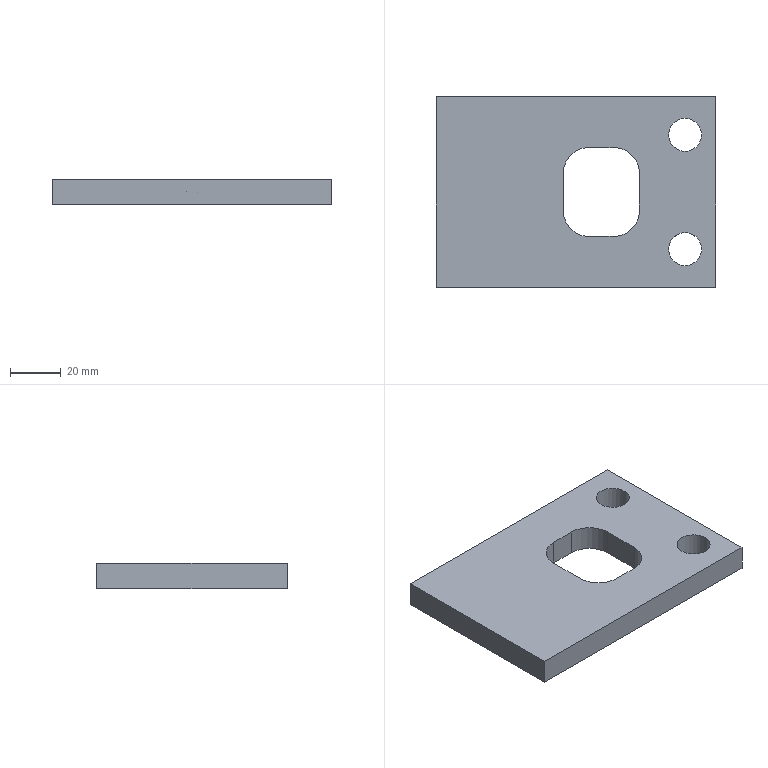Part | NX | features solid 2 | 1 solid | 16 faces | box 110 x 75 x 10 mm | volume 70204 mm3 | plane 10 | cylinder 6 | commonest cylinder face diameters 20 x4 13 x2
STEP:
#1=CARTESIAN_POINT('',(373.,202.5,-55.));
#2=VERTEX_POINT('',#1);
#3=CARTESIAN_POINT('',(363.,202.5,-55.));
#4=VERTEX_POINT('',#3);
#5=CARTESIAN_POINT('',(316.,202.5,-55.));
#6=DIRECTION('',(-1.,0.,0.));
#7=VECTOR('',#6,1000.);
#8=LINE('',#5,#7);
#9=EDGE_CURVE('',#2,#4,#8,.T.);
#10=ORIENTED_EDGE('',*,*,#9,.F.);
#11=CARTESIAN_POINT('',(373.,202.5,-45.));
#12=VERTEX_POINT('',#11);
#13=CARTESIAN_POINT('',(373.,202.5,-45.));
#14=DIRECTION('',(0.,0.,-1.));
#15=VECTOR('',#14,1000.);
#16=LINE('',#13,#15);
#17=EDGE_CURVE('',#2,#12,#16,.F.);
#18=ORIENTED_EDGE('',*,*,#17,.T.);
#19=CARTESIAN_POINT('',(363.,202.5,-45.));
#20=VERTEX_POINT('',#19);
#21=CARTESIAN_POINT('',(316.,202.5,-45.));
#22=DIRECTION('',(-1.,0.,0.));
#23=VECTOR('',#22,1000.);
#24=LINE('',#21,#23);
#25=EDGE_CURVE('',#12,#20,#24,.T.);
#26=ORIENTED_EDGE('',*,*,#25,.T.);
#27=CARTESIAN_POINT('',(363.,202.5,-55.));
#28=DIRECTION('',(0.,0.,1.));
#29=VECTOR('',#28,1000.);
#30=LINE('',#27,#29);
#31=EDGE_CURVE('',#20,#4,#30,.F.);
#32=ORIENTED_EDGE('',*,*,#31,.T.);
#33=EDGE_LOOP('',(#10,#18,#26,#32));
#34=FACE_BOUND('',#33,.T.);
#35=CARTESIAN_POINT('',(301.,202.5,-111.));
#36=DIRECTION('',(0.,1.,0.));
#37=DIRECTION('',(0.,0.,-1.));
#38=AXIS2_PLACEMENT_3D('',#35,#36,#37);
#39=PLANE('',#38);
#40=ADVANCED_FACE('',(#34),#39,.F.);
#41=CARTESIAN_POINT('',(353.,192.5,-55.));
#42=VERTEX_POINT('',#41);
#43=CARTESIAN_POINT('',(363.,192.5,-55.));
#44=DIRECTION('',(0.,0.,1.));
#45=DIRECTION('',(0.,1.,0.));
#46=AXIS2_PLACEMENT_3D('',#43,#44,#45);
#47=CIRCLE('',#46,10.);
#48=EDGE_CURVE('',#4,#42,#47,.T.);
#49=ORIENTED_EDGE('',*,*,#48,.T.);
#50=CARTESIAN_POINT('',(353.,177.5,-55.));
#51=VERTEX_POINT('',#50);
#52=CARTESIAN_POINT('',(353.,185.,-55.));
#53=DIRECTION('',(0.,-1.,0.));
#54=VECTOR('',#53,1000.);
#55=LINE('',#52,#54);
#56=EDGE_CURVE('',#42,#51,#55,.T.);
#57=ORIENTED_EDGE('',*,*,#56,.T.);
#58=CARTESIAN_POINT('',(363.,167.5,-55.));
#59=VERTEX_POINT('',#58);
#60=CARTESIAN_POINT('',(363.,177.5,-55.));
#61=DIRECTION('',(0.,0.,1.));
#62=DIRECTION('',(0.,1.,0.));
#63=AXIS2_PLACEMENT_3D('',#60,#61,#62);
#64=CIRCLE('',#63,10.);
#65=EDGE_CURVE('',#51,#59,#64,.T.);
#66=ORIENTED_EDGE('',*,*,#65,.T.);
#67=CARTESIAN_POINT('',(373.,167.5,-55.));
#68=VERTEX_POINT('',#67);
#69=CARTESIAN_POINT('',(316.,167.5,-55.));
#70=DIRECTION('',(-1.,0.,0.));
#71=VECTOR('',#70,1000.);
#72=LINE('',#69,#71);
#73=EDGE_CURVE('',#68,#59,#72,.T.);
#74=ORIENTED_EDGE('',*,*,#73,.F.);
#75=CARTESIAN_POINT('',(383.,177.5,-55.));
#76=VERTEX_POINT('',#75);
#77=CARTESIAN_POINT('',(373.,177.5,-55.));
#78=DIRECTION('',(0.,0.,1.));
#79=DIRECTION('',(0.,1.,0.));
#80=AXIS2_PLACEMENT_3D('',#77,#78,#79);
#81=CIRCLE('',#80,10.);
#82=EDGE_CURVE('',#68,#76,#81,.T.);
#83=ORIENTED_EDGE('',*,*,#82,.T.);
#84=CARTESIAN_POINT('',(383.,192.5,-55.));
#85=VERTEX_POINT('',#84);
#86=CARTESIAN_POINT('',(383.,140.,-55.));
#87=DIRECTION('',(0.,-1.,0.));
#88=VECTOR('',#87,1000.);
#89=LINE('',#86,#88);
#90=EDGE_CURVE('',#76,#85,#89,.F.);
#91=ORIENTED_EDGE('',*,*,#90,.T.);
#92=CARTESIAN_POINT('',(373.,192.5,-55.));
#93=DIRECTION('',(0.,0.,1.));
#94=DIRECTION('',(0.,1.,0.));
#95=AXIS2_PLACEMENT_3D('',#92,#93,#94);
#96=CIRCLE('',#95,10.);
#97=EDGE_CURVE('',#85,#2,#96,.T.);
#98=ORIENTED_EDGE('',*,*,#97,.T.);
#99=ORIENTED_EDGE('',*,*,#9,.T.);
#100=EDGE_LOOP('',(#49,#57,#66,#74,#83,#91,#98,#99));
#101=FACE_BOUND('',#100,.T.);
#102=CARTESIAN_POINT('',(413.,222.5,-55.));
#103=VERTEX_POINT('',#102);
#104=CARTESIAN_POINT('',(303.,222.5,-55.));
#105=VERTEX_POINT('',#104);
#106=CARTESIAN_POINT('',(316.,222.5,-55.));
#107=DIRECTION('',(1.,0.,0.));
#108=VECTOR('',#107,1000.);
#109=LINE('',#106,#108);
#110=EDGE_CURVE('',#103,#105,#109,.F.);
#111=ORIENTED_EDGE('',*,*,#110,.F.);
#112=CARTESIAN_POINT('',(413.,147.5,-55.));
#113=VERTEX_POINT('',#112);
#114=CARTESIAN_POINT('',(413.,140.,-55.));
#115=DIRECTION('',(0.,-1.,0.));
#116=VECTOR('',#115,1000.);
#117=LINE('',#114,#116);
#118=EDGE_CURVE('',#113,#103,#117,.F.);
#119=ORIENTED_EDGE('',*,*,#118,.F.);
#120=CARTESIAN_POINT('',(303.,147.5,-55.));
#121=VERTEX_POINT('',#120);
#122=CARTESIAN_POINT('',(316.,147.5,-55.));
#123=DIRECTION('',(1.,0.,0.));
#124=VECTOR('',#123,1000.);
#125=LINE('',#122,#124);
#126=EDGE_CURVE('',#113,#121,#125,.F.);
#127=ORIENTED_EDGE('',*,*,#126,.T.);
#128=CARTESIAN_POINT('',(303.,140.,-55.));
#129=DIRECTION('',(0.,1.,0.));
#130=VECTOR('',#129,1000.);
#131=LINE('',#128,#130);
#132=EDGE_CURVE('',#121,#105,#131,.T.);
#133=ORIENTED_EDGE('',*,*,#132,.T.);
#134=EDGE_LOOP('',(#111,#119,#127,#133));
#135=FACE_BOUND('',#134,.T.);
#136=CARTESIAN_POINT('',(401.,169.,-55.));
#137=VERTEX_POINT('',#136);
#138=CARTESIAN_POINT('',(401.,162.5,-55.));
#139=DIRECTION('',(0.,0.,-1.));
#140=DIRECTION('',(0.,1.,0.));
#141=AXIS2_PLACEMENT_3D('',#138,#139,#140);
#142=CIRCLE('',#141,6.5);
#143=EDGE_CURVE('',#137,#137,#142,.F.);
#144=ORIENTED_EDGE('',*,*,#143,.T.);
#145=EDGE_LOOP('',(#144));
#146=FACE_BOUND('',#145,.T.);
#147=CARTESIAN_POINT('',(401.,214.,-55.));
#148=VERTEX_POINT('',#147);
#149=CARTESIAN_POINT('',(401.,207.5,-55.));
#150=DIRECTION('',(0.,0.,-1.));
#151=DIRECTION('',(0.,1.,0.));
#152=AXIS2_PLACEMENT_3D('',#149,#150,#151);
#153=CIRCLE('',#152,6.5);
#154=EDGE_CURVE('',#148,#148,#153,.T.);
#155=ORIENTED_EDGE('',*,*,#154,.F.);
#156=EDGE_LOOP('',(#155));
#157=FACE_BOUND('',#156,.T.);
#158=CARTESIAN_POINT('',(316.,140.,-55.));
#159=DIRECTION('',(0.,0.,1.));
#160=DIRECTION('',(0.,1.,0.));
#161=AXIS2_PLACEMENT_3D('',#158,#159,#160);
#162=PLANE('',#161);
#163=ADVANCED_FACE('',(#101,#135,#146,#157),#162,.F.);
#164=ORIENTED_EDGE('',*,*,#25,.F.);
#165=CARTESIAN_POINT('',(383.,192.5,-45.));
#166=VERTEX_POINT('',#165);
#167=CARTESIAN_POINT('',(373.,192.5,-45.));
#168=DIRECTION('',(0.,0.,1.));
#169=DIRECTION('',(0.,1.,0.));
#170=AXIS2_PLACEMENT_3D('',#167,#168,#169);
#171=CIRCLE('',#170,10.);
#172=EDGE_CURVE('',#12,#166,#171,.F.);
#173=ORIENTED_EDGE('',*,*,#172,.T.);
#174=CARTESIAN_POINT('',(383.,177.5,-45.));
#175=VERTEX_POINT('',#174);
#176=CARTESIAN_POINT('',(383.,140.,-45.));
#177=DIRECTION('',(0.,-1.,0.));
#178=VECTOR('',#177,1000.);
#179=LINE('',#176,#178);
#180=EDGE_CURVE('',#175,#166,#179,.F.);
#181=ORIENTED_EDGE('',*,*,#180,.F.);
#182=CARTESIAN_POINT('',(373.,167.5,-45.));
#183=VERTEX_POINT('',#182);
#184=CARTESIAN_POINT('',(373.,177.5,-45.));
#185=DIRECTION('',(0.,0.,1.));
#186=DIRECTION('',(0.,1.,0.));
#187=AXIS2_PLACEMENT_3D('',#184,#185,#186);
#188=CIRCLE('',#187,10.);
#189=EDGE_CURVE('',#175,#183,#188,.F.);
#190=ORIENTED_EDGE('',*,*,#189,.T.);
#191=CARTESIAN_POINT('',(363.,167.5,-45.));
#192=VERTEX_POINT('',#191);
#193=CARTESIAN_POINT('',(316.,167.5,-45.));
#194=DIRECTION('',(-1.,0.,0.));
#195=VECTOR('',#194,1000.);
#196=LINE('',#193,#195);
#197=EDGE_CURVE('',#183,#192,#196,.T.);
#198=ORIENTED_EDGE('',*,*,#197,.T.);
#199=CARTESIAN_POINT('',(353.,177.5,-45.));
#200=VERTEX_POINT('',#199);
#201=CARTESIAN_POINT('',(363.,177.5,-45.));
#202=DIRECTION('',(0.,0.,1.));
#203=DIRECTION('',(0.,1.,0.));
#204=AXIS2_PLACEMENT_3D('',#201,#202,#203);
#205=CIRCLE('',#204,10.);
#206=EDGE_CURVE('',#192,#200,#205,.F.);
#207=ORIENTED_EDGE('',*,*,#206,.T.);
#208=CARTESIAN_POINT('',(353.,192.5,-45.));
#209=VERTEX_POINT('',#208);
#210=CARTESIAN_POINT('',(353.,140.,-45.));
#211=DIRECTION('',(0.,1.,0.));
#212=VECTOR('',#211,1000.);
#213=LINE('',#210,#212);
#214=EDGE_CURVE('',#200,#209,#213,.T.);
#215=ORIENTED_EDGE('',*,*,#214,.T.);
#216=CARTESIAN_POINT('',(363.,192.5,-45.));
#217=DIRECTION('',(0.,0.,1.));
#218=DIRECTION('',(0.,1.,0.));
#219=AXIS2_PLACEMENT_3D('',#216,#217,#218);
#220=CIRCLE('',#219,10.);
#221=EDGE_CURVE('',#209,#20,#220,.F.);
#222=ORIENTED_EDGE('',*,*,#221,.T.);
#223=EDGE_LOOP('',(#164,#173,#181,#190,#198,#207,#215,#222));
#224=FACE_BOUND('',#223,.T.);
#225=CARTESIAN_POINT('',(303.,147.5,-45.));
#226=VERTEX_POINT('',#225);
#227=CARTESIAN_POINT('',(303.,222.5,-45.));
#228=VERTEX_POINT('',#227);
#229=CARTESIAN_POINT('',(303.,140.,-45.));
#230=DIRECTION('',(0.,1.,0.));
#231=VECTOR('',#230,1000.);
#232=LINE('',#229,#231);
#233=EDGE_CURVE('',#226,#228,#232,.T.);
#234=ORIENTED_EDGE('',*,*,#233,.F.);
#235=CARTESIAN_POINT('',(413.,147.5,-45.));
#236=VERTEX_POINT('',#235);
#237=CARTESIAN_POINT('',(316.,147.5,-45.));
#238=DIRECTION('',(1.,0.,0.));
#239=VECTOR('',#238,1000.);
#240=LINE('',#237,#239);
#241=EDGE_CURVE('',#236,#226,#240,.F.);
#242=ORIENTED_EDGE('',*,*,#241,.F.);
#243=CARTESIAN_POINT('',(413.,222.5,-45.));
#244=VERTEX_POINT('',#243);
#245=CARTESIAN_POINT('',(413.,140.,-45.));
#246=DIRECTION('',(0.,-1.,0.));
#247=VECTOR('',#246,1000.);
#248=LINE('',#245,#247);
#249=EDGE_CURVE('',#236,#244,#248,.F.);
#250=ORIENTED_EDGE('',*,*,#249,.T.);
#251=CARTESIAN_POINT('',(316.,222.5,-45.));
#252=DIRECTION('',(1.,0.,0.));
#253=VECTOR('',#252,1000.);
#254=LINE('',#251,#253);
#255=EDGE_CURVE('',#244,#228,#254,.F.);
#256=ORIENTED_EDGE('',*,*,#255,.T.);
#257=EDGE_LOOP('',(#234,#242,#250,#256));
#258=FACE_BOUND('',#257,.T.);
#259=CARTESIAN_POINT('',(401.,169.,-45.));
#260=VERTEX_POINT('',#259);
#261=CARTESIAN_POINT('',(401.,162.5,-45.));
#262=DIRECTION('',(0.,0.,-1.));
#263=DIRECTION('',(0.,1.,0.));
#264=AXIS2_PLACEMENT_3D('',#261,#262,#263);
#265=CIRCLE('',#264,6.5);
#266=EDGE_CURVE('',#260,#260,#265,.F.);
#267=ORIENTED_EDGE('',*,*,#266,.F.);
#268=EDGE_LOOP('',(#267));
#269=FACE_BOUND('',#268,.T.);
#270=CARTESIAN_POINT('',(401.,214.,-45.));
#271=VERTEX_POINT('',#270);
#272=CARTESIAN_POINT('',(401.,207.5,-45.));
#273=DIRECTION('',(0.,0.,-1.));
#274=DIRECTION('',(0.,1.,0.));
#275=AXIS2_PLACEMENT_3D('',#272,#273,#274);
#276=CIRCLE('',#275,6.5);
#277=EDGE_CURVE('',#271,#271,#276,.T.);
#278=ORIENTED_EDGE('',*,*,#277,.T.);
#279=EDGE_LOOP('',(#278));
#280=FACE_BOUND('',#279,.T.);
#281=CARTESIAN_POINT('',(316.,140.,-45.));
#282=DIRECTION('',(0.,0.,1.));
#283=DIRECTION('',(0.,1.,0.));
#284=AXIS2_PLACEMENT_3D('',#281,#282,#283);
#285=PLANE('',#284);
#286=ADVANCED_FACE('',(#224,#258,#269,#280),#285,.T.);
#287=ORIENTED_EDGE('',*,*,#249,.F.);
#288=CARTESIAN_POINT('',(413.,147.5,-55.));
#289=DIRECTION('',(0.,0.,-1.));
#290=VECTOR('',#289,1000.);
#291=LINE('',#288,#290);
#292=EDGE_CURVE('',#236,#113,#291,.T.);
#293=ORIENTED_EDGE('',*,*,#292,.T.);
#294=ORIENTED_EDGE('',*,*,#118,.T.);
#295=CARTESIAN_POINT('',(413.,222.5,-55.));
#296=DIRECTION('',(0.,0.,1.));
#297=VECTOR('',#296,1000.);
#298=LINE('',#295,#297);
#299=EDGE_CURVE('',#103,#244,#298,.T.);
#300=ORIENTED_EDGE('',*,*,#299,.T.);
#301=EDGE_LOOP('',(#287,#293,#294,#300));
#302=FACE_BOUND('',#301,.T.);
#303=CARTESIAN_POINT('',(413.,140.,-55.));
#304=DIRECTION('',(1.,0.,0.));
#305=DIRECTION('',(0.,1.,0.));
#306=AXIS2_PLACEMENT_3D('',#303,#304,#305);
#307=PLANE('',#306);
#308=ADVANCED_FACE('',(#302),#307,.T.);
#309=ORIENTED_EDGE('',*,*,#255,.F.);
#310=ORIENTED_EDGE('',*,*,#299,.F.);
#311=ORIENTED_EDGE('',*,*,#110,.T.);
#312=CARTESIAN_POINT('',(303.,222.5,-55.));
#313=DIRECTION('',(0.,0.,1.));
#314=VECTOR('',#313,1000.);
#315=LINE('',#312,#314);
#316=EDGE_CURVE('',#228,#105,#315,.F.);
#317=ORIENTED_EDGE('',*,*,#316,.F.);
#318=EDGE_LOOP('',(#309,#310,#311,#317));
#319=FACE_BOUND('',#318,.T.);
#320=CARTESIAN_POINT('',(316.,222.5,-55.));
#321=DIRECTION('',(0.,1.,0.));
#322=DIRECTION('',(-1.,0.,0.));
#323=AXIS2_PLACEMENT_3D('',#320,#321,#322);
#324=PLANE('',#323);
#325=ADVANCED_FACE('',(#319),#324,.T.);
#326=ORIENTED_EDGE('',*,*,#126,.F.);
#327=ORIENTED_EDGE('',*,*,#292,.F.);
#328=ORIENTED_EDGE('',*,*,#241,.T.);
#329=CARTESIAN_POINT('',(303.,147.5,-55.));
#330=DIRECTION('',(0.,0.,-1.));
#331=VECTOR('',#330,1000.);
#332=LINE('',#329,#331);
#333=EDGE_CURVE('',#121,#226,#332,.F.);
#334=ORIENTED_EDGE('',*,*,#333,.F.);
#335=EDGE_LOOP('',(#326,#327,#328,#334));
#336=FACE_BOUND('',#335,.T.);
#337=CARTESIAN_POINT('',(586.,147.5,-55.));
#338=DIRECTION('',(0.,-1.,0.));
#339=DIRECTION('',(0.,0.,1.));
#340=AXIS2_PLACEMENT_3D('',#337,#338,#339);
#341=PLANE('',#340);
#342=ADVANCED_FACE('',(#336),#341,.T.);
#343=ORIENTED_EDGE('',*,*,#266,.T.);
#344=EDGE_LOOP('',(#343));
#345=FACE_BOUND('',#344,.T.);
#346=ORIENTED_EDGE('',*,*,#143,.F.);
#347=EDGE_LOOP('',(#346));
#348=FACE_BOUND('',#347,.T.);
#349=CARTESIAN_POINT('',(401.,162.5,-174.));
#350=DIRECTION('',(0.,0.,1.));
#351=DIRECTION('',(0.,1.,0.));
#352=AXIS2_PLACEMENT_3D('',#349,#350,#351);
#353=CYLINDRICAL_SURFACE('',#352,6.5);
#354=ADVANCED_FACE('',(#345,#348),#353,.F.);
#355=ORIENTED_EDGE('',*,*,#277,.F.);
#356=EDGE_LOOP('',(#355));
#357=FACE_BOUND('',#356,.T.);
#358=ORIENTED_EDGE('',*,*,#154,.T.);
#359=EDGE_LOOP('',(#358));
#360=FACE_BOUND('',#359,.T.);
#361=CARTESIAN_POINT('',(401.,207.5,-174.));
#362=DIRECTION('',(0.,0.,1.));
#363=DIRECTION('',(0.,1.,0.));
#364=AXIS2_PLACEMENT_3D('',#361,#362,#363);
#365=CYLINDRICAL_SURFACE('',#364,6.5);
#366=ADVANCED_FACE('',(#357,#360),#365,.F.);
#367=ORIENTED_EDGE('',*,*,#180,.T.);
#368=CARTESIAN_POINT('',(383.,192.5,-55.));
#369=DIRECTION('',(0.,0.,1.));
#370=VECTOR('',#369,1000.);
#371=LINE('',#368,#370);
#372=EDGE_CURVE('',#166,#85,#371,.F.);
#373=ORIENTED_EDGE('',*,*,#372,.T.);
#374=ORIENTED_EDGE('',*,*,#90,.F.);
#375=CARTESIAN_POINT('',(383.,177.5,-111.));
#376=DIRECTION('',(0.,0.,1.));
#377=VECTOR('',#376,1000.);
#378=LINE('',#375,#377);
#379=EDGE_CURVE('',#76,#175,#378,.T.);
#380=ORIENTED_EDGE('',*,*,#379,.T.);
#381=EDGE_LOOP('',(#367,#373,#374,#380));
#382=FACE_BOUND('',#381,.T.);
#383=CARTESIAN_POINT('',(383.,185.,-111.));
#384=DIRECTION('',(-1.,0.,0.));
#385=DIRECTION('',(0.,0.,1.));
#386=AXIS2_PLACEMENT_3D('',#383,#384,#385);
#387=PLANE('',#386);
#388=ADVANCED_FACE('',(#382),#387,.T.);
#389=ORIENTED_EDGE('',*,*,#197,.F.);
#390=CARTESIAN_POINT('',(373.,167.5,-111.));
#391=DIRECTION('',(0.,0.,-1.));
#392=VECTOR('',#391,1000.);
#393=LINE('',#390,#392);
#394=EDGE_CURVE('',#183,#68,#393,.T.);
#395=ORIENTED_EDGE('',*,*,#394,.T.);
#396=ORIENTED_EDGE('',*,*,#73,.T.);
#397=CARTESIAN_POINT('',(363.,167.5,-111.));
#398=DIRECTION('',(0.,0.,1.));
#399=VECTOR('',#398,1000.);
#400=LINE('',#397,#399);
#401=EDGE_CURVE('',#59,#192,#400,.T.);
#402=ORIENTED_EDGE('',*,*,#401,.T.);
#403=EDGE_LOOP('',(#389,#395,#396,#402));
#404=FACE_BOUND('',#403,.T.);
#405=CARTESIAN_POINT('',(301.,167.5,-111.));
#406=DIRECTION('',(0.,1.,0.));
#407=DIRECTION('',(0.,0.,-1.));
#408=AXIS2_PLACEMENT_3D('',#405,#406,#407);
#409=PLANE('',#408);
#410=ADVANCED_FACE('',(#404),#409,.T.);
#411=ORIENTED_EDGE('',*,*,#82,.F.);
#412=ORIENTED_EDGE('',*,*,#394,.F.);
#413=ORIENTED_EDGE('',*,*,#189,.F.);
#414=ORIENTED_EDGE('',*,*,#379,.F.);
#415=EDGE_LOOP('',(#411,#412,#413,#414));
#416=FACE_BOUND('',#415,.T.);
#417=CARTESIAN_POINT('',(373.,177.5,-111.));
#418=DIRECTION('',(0.,0.,-1.));
#419=DIRECTION('',(0.,-1.,0.));
#420=AXIS2_PLACEMENT_3D('',#417,#418,#419);
#421=CYLINDRICAL_SURFACE('',#420,10.);
#422=ADVANCED_FACE('',(#416),#421,.F.);
#423=ORIENTED_EDGE('',*,*,#97,.F.);
#424=ORIENTED_EDGE('',*,*,#372,.F.);
#425=ORIENTED_EDGE('',*,*,#172,.F.);
#426=ORIENTED_EDGE('',*,*,#17,.F.);
#427=EDGE_LOOP('',(#423,#424,#425,#426));
#428=FACE_BOUND('',#427,.T.);
#429=CARTESIAN_POINT('',(373.,192.5,-111.));
#430=DIRECTION('',(0.,0.,1.));
#431=DIRECTION('',(0.,1.,0.));
#432=AXIS2_PLACEMENT_3D('',#429,#430,#431);
#433=CYLINDRICAL_SURFACE('',#432,10.);
#434=ADVANCED_FACE('',(#428),#433,.F.);
#435=ORIENTED_EDGE('',*,*,#56,.F.);
#436=CARTESIAN_POINT('',(353.,192.5,-45.));
#437=DIRECTION('',(0.,0.,1.));
#438=VECTOR('',#437,1000.);
#439=LINE('',#436,#438);
#440=EDGE_CURVE('',#42,#209,#439,.T.);
#441=ORIENTED_EDGE('',*,*,#440,.T.);
#442=ORIENTED_EDGE('',*,*,#214,.F.);
#443=CARTESIAN_POINT('',(353.,177.5,-111.));
#444=DIRECTION('',(0.,0.,1.));
#445=VECTOR('',#444,1000.);
#446=LINE('',#443,#445);
#447=EDGE_CURVE('',#200,#51,#446,.F.);
#448=ORIENTED_EDGE('',*,*,#447,.T.);
#449=EDGE_LOOP('',(#435,#441,#442,#448));
#450=FACE_BOUND('',#449,.T.);
#451=CARTESIAN_POINT('',(353.,185.,-111.));
#452=DIRECTION('',(-1.,0.,0.));
#453=DIRECTION('',(0.,0.,1.));
#454=AXIS2_PLACEMENT_3D('',#451,#452,#453);
#455=PLANE('',#454);
#456=ADVANCED_FACE('',(#450),#455,.F.);
#457=ORIENTED_EDGE('',*,*,#132,.F.);
#458=ORIENTED_EDGE('',*,*,#333,.T.);
#459=ORIENTED_EDGE('',*,*,#233,.T.);
#460=ORIENTED_EDGE('',*,*,#316,.T.);
#461=EDGE_LOOP('',(#457,#458,#459,#460));
#462=FACE_BOUND('',#461,.T.);
#463=CARTESIAN_POINT('',(303.,140.,-55.));
#464=DIRECTION('',(1.,0.,0.));
#465=DIRECTION('',(0.,1.,0.));
#466=AXIS2_PLACEMENT_3D('',#463,#464,#465);
#467=PLANE('',#466);
#468=ADVANCED_FACE('',(#462),#467,.F.);
#469=ORIENTED_EDGE('',*,*,#48,.F.);
#470=ORIENTED_EDGE('',*,*,#31,.F.);
#471=ORIENTED_EDGE('',*,*,#221,.F.);
#472=ORIENTED_EDGE('',*,*,#440,.F.);
#473=EDGE_LOOP('',(#469,#470,#471,#472));
#474=FACE_BOUND('',#473,.T.);
#475=CARTESIAN_POINT('',(363.,192.5,-111.));
#476=DIRECTION('',(0.,0.,-1.));
#477=DIRECTION('',(0.,-1.,0.));
#478=AXIS2_PLACEMENT_3D('',#475,#476,#477);
#479=CYLINDRICAL_SURFACE('',#478,10.);
#480=ADVANCED_FACE('',(#474),#479,.F.);
#481=ORIENTED_EDGE('',*,*,#65,.F.);
#482=ORIENTED_EDGE('',*,*,#447,.F.);
#483=ORIENTED_EDGE('',*,*,#206,.F.);
#484=ORIENTED_EDGE('',*,*,#401,.F.);
#485=EDGE_LOOP('',(#481,#482,#483,#484));
#486=FACE_BOUND('',#485,.T.);
#487=CARTESIAN_POINT('',(363.,177.5,-111.));
#488=DIRECTION('',(0.,0.,1.));
#489=DIRECTION('',(0.,1.,0.));
#490=AXIS2_PLACEMENT_3D('',#487,#488,#489);
#491=CYLINDRICAL_SURFACE('',#490,10.);
#492=ADVANCED_FACE('',(#486),#491,.F.);
#493=CLOSED_SHELL('',(#40,#163,#286,#308,#325,#342,#354,#366,#388,#410,#422,#434,#456,#468,#480,#492));
#494=MANIFOLD_SOLID_BREP('',#493);
#495=(LENGTH_UNIT()NAMED_UNIT(*)SI_UNIT(.MILLI.,.METRE.));
#496=UNCERTAINTY_MEASURE_WITH_UNIT(LENGTH_MEASURE(0.00001),#495,'','');
#497=(NAMED_UNIT(*)PLANE_ANGLE_UNIT()SI_UNIT($,.RADIAN.));
#498=(NAMED_UNIT(*)SI_UNIT($,.STERADIAN.)SOLID_ANGLE_UNIT());
#499=(GEOMETRIC_REPRESENTATION_CONTEXT(3)GLOBAL_UNCERTAINTY_ASSIGNED_CONTEXT((#496))GLOBAL_UNIT_ASSIGNED_CONTEXT((#495,#497,#498))REPRESENTATION_CONTEXT('',''));
#500=ADVANCED_BREP_SHAPE_REPRESENTATION('',(#494),#499);